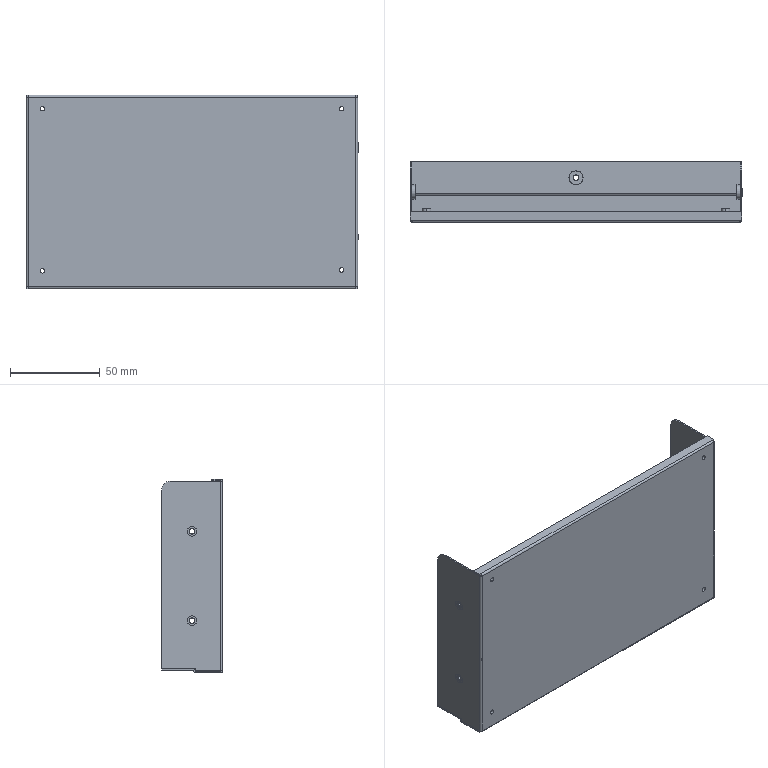Part | SolidWorks | features BaseBody 6 | 6 solids | 137 faces | box 185.4 x 34 x 108 mm | volume 28122 mm3 | cylinder 70 | plane 57 | spline 10 | commonest cylinder face diameters 3 x10 3.3 x10 5.4 x10 8 x10 2.5 x8 5 x8